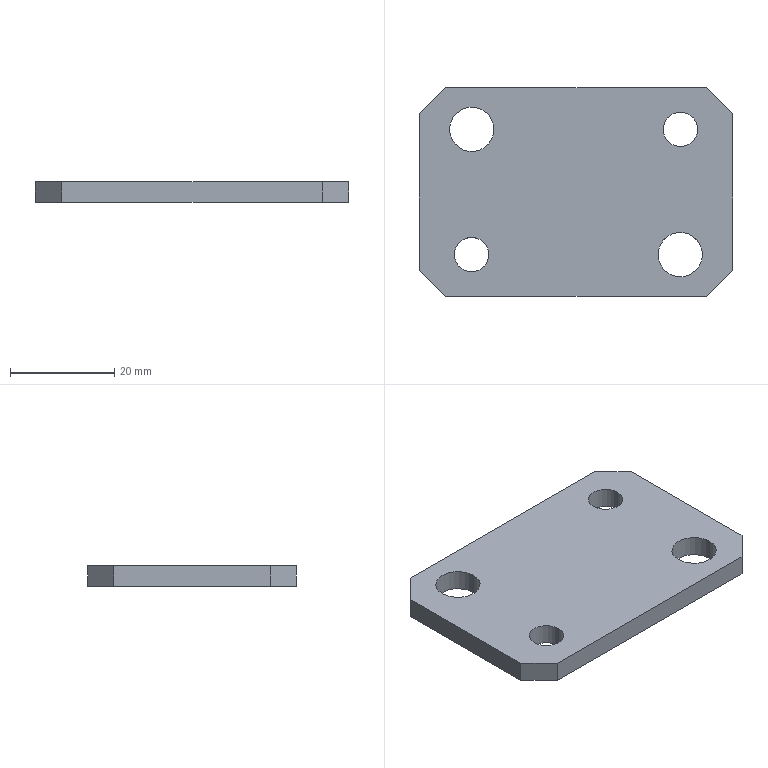Part | SolidWorks | features Chamfer 1, Extrusion 1 | 1 solid | 18 faces | box 60 x 40 x 4 mm | volume 8672 mm3 | plane 10 | cylinder 8 | commonest cylinder face diameters 6.6 x4 8.5 x4
STEP:
#1=CARTESIAN_POINT('',(-18.291,-17.534,4.));
#2=VERTEX_POINT('',#1);
#3=CARTESIAN_POINT('',(-11.691,-17.534,4.));
#4=VERTEX_POINT('',#3);
#5=CARTESIAN_POINT('',(-14.991,-17.534,4.));
#6=DIRECTION('',(0.,0.,1.));
#7=DIRECTION('',(1.,0.,0.));
#8=AXIS2_PLACEMENT_3D('',#5,#6,#7);
#9=CIRCLE('',#8,3.3);
#10=EDGE_CURVE('',#2,#4,#9,.T.);
#11=ORIENTED_EDGE('',*,*,#10,.T.);
#12=CARTESIAN_POINT('',(-11.691,-17.534,0.));
#13=VERTEX_POINT('',#12);
#14=CARTESIAN_POINT('',(-11.691,-17.534,4.));
#15=DIRECTION('',(0.,0.,-1.));
#16=VECTOR('',#15,1000.);
#17=LINE('',#14,#16);
#18=EDGE_CURVE('',#4,#13,#17,.T.);
#19=ORIENTED_EDGE('',*,*,#18,.T.);
#20=CARTESIAN_POINT('',(-18.291,-17.534,0.));
#21=VERTEX_POINT('',#20);
#22=CARTESIAN_POINT('',(-14.991,-17.534,0.));
#23=DIRECTION('',(0.,0.,1.));
#24=DIRECTION('',(1.,0.,0.));
#25=AXIS2_PLACEMENT_3D('',#22,#23,#24);
#26=CIRCLE('',#25,3.3);
#27=EDGE_CURVE('',#21,#13,#26,.T.);
#28=ORIENTED_EDGE('',*,*,#27,.F.);
#29=CARTESIAN_POINT('',(-18.291,-17.534,4.));
#30=DIRECTION('',(0.,0.,-1.));
#31=VECTOR('',#30,1000.);
#32=LINE('',#29,#31);
#33=EDGE_CURVE('',#2,#21,#32,.T.);
#34=ORIENTED_EDGE('',*,*,#33,.F.);
#35=EDGE_LOOP('',(#11,#19,#28,#34));
#36=FACE_OUTER_BOUND('',#35,.T.);
#37=CARTESIAN_POINT('',(-14.991,-17.534,4.));
#38=DIRECTION('',(0.,0.,-1.));
#39=DIRECTION('',(-1.,0.,0.));
#40=AXIS2_PLACEMENT_3D('',#37,#38,#39);
#41=CYLINDRICAL_SURFACE('',#40,3.3);
#42=ADVANCED_FACE('',(#36),#41,.F.);
#43=CARTESIAN_POINT('',(21.709,6.466,4.));
#44=VERTEX_POINT('',#43);
#45=CARTESIAN_POINT('',(28.309,6.466,4.));
#46=VERTEX_POINT('',#45);
#47=CARTESIAN_POINT('',(25.009,6.466,4.));
#48=DIRECTION('',(0.,0.,1.));
#49=DIRECTION('',(1.,0.,0.));
#50=AXIS2_PLACEMENT_3D('',#47,#48,#49);
#51=CIRCLE('',#50,3.3);
#52=EDGE_CURVE('',#44,#46,#51,.T.);
#53=ORIENTED_EDGE('',*,*,#52,.T.);
#54=CARTESIAN_POINT('',(28.309,6.466,0.));
#55=VERTEX_POINT('',#54);
#56=CARTESIAN_POINT('',(28.309,6.466,4.));
#57=DIRECTION('',(0.,0.,-1.));
#58=VECTOR('',#57,1000.);
#59=LINE('',#56,#58);
#60=EDGE_CURVE('',#46,#55,#59,.T.);
#61=ORIENTED_EDGE('',*,*,#60,.T.);
#62=CARTESIAN_POINT('',(21.709,6.466,0.));
#63=VERTEX_POINT('',#62);
#64=CARTESIAN_POINT('',(25.009,6.466,0.));
#65=DIRECTION('',(0.,0.,1.));
#66=DIRECTION('',(1.,0.,0.));
#67=AXIS2_PLACEMENT_3D('',#64,#65,#66);
#68=CIRCLE('',#67,3.3);
#69=EDGE_CURVE('',#63,#55,#68,.T.);
#70=ORIENTED_EDGE('',*,*,#69,.F.);
#71=CARTESIAN_POINT('',(21.709,6.466,4.));
#72=DIRECTION('',(0.,0.,-1.));
#73=VECTOR('',#72,1000.);
#74=LINE('',#71,#73);
#75=EDGE_CURVE('',#44,#63,#74,.T.);
#76=ORIENTED_EDGE('',*,*,#75,.F.);
#77=EDGE_LOOP('',(#53,#61,#70,#76));
#78=FACE_OUTER_BOUND('',#77,.T.);
#79=CARTESIAN_POINT('',(25.009,6.466,4.));
#80=DIRECTION('',(0.,0.,-1.));
#81=DIRECTION('',(-1.,0.,0.));
#82=AXIS2_PLACEMENT_3D('',#79,#80,#81);
#83=CYLINDRICAL_SURFACE('',#82,3.3);
#84=ADVANCED_FACE('',(#78),#83,.F.);
#85=CARTESIAN_POINT('',(20.759,-17.534,4.));
#86=VERTEX_POINT('',#85);
#87=CARTESIAN_POINT('',(29.259,-17.534,4.));
#88=VERTEX_POINT('',#87);
#89=CARTESIAN_POINT('',(25.009,-17.534,4.));
#90=DIRECTION('',(0.,0.,1.));
#91=DIRECTION('',(1.,0.,0.));
#92=AXIS2_PLACEMENT_3D('',#89,#90,#91);
#93=CIRCLE('',#92,4.25);
#94=EDGE_CURVE('',#86,#88,#93,.T.);
#95=ORIENTED_EDGE('',*,*,#94,.T.);
#96=CARTESIAN_POINT('',(29.259,-17.534,0.));
#97=VERTEX_POINT('',#96);
#98=CARTESIAN_POINT('',(29.259,-17.534,4.));
#99=DIRECTION('',(0.,0.,-1.));
#100=VECTOR('',#99,1000.);
#101=LINE('',#98,#100);
#102=EDGE_CURVE('',#88,#97,#101,.T.);
#103=ORIENTED_EDGE('',*,*,#102,.T.);
#104=CARTESIAN_POINT('',(20.759,-17.534,0.));
#105=VERTEX_POINT('',#104);
#106=CARTESIAN_POINT('',(25.009,-17.534,0.));
#107=DIRECTION('',(0.,0.,1.));
#108=DIRECTION('',(1.,0.,0.));
#109=AXIS2_PLACEMENT_3D('',#106,#107,#108);
#110=CIRCLE('',#109,4.25);
#111=EDGE_CURVE('',#105,#97,#110,.T.);
#112=ORIENTED_EDGE('',*,*,#111,.F.);
#113=CARTESIAN_POINT('',(20.759,-17.534,4.));
#114=DIRECTION('',(0.,0.,-1.));
#115=VECTOR('',#114,1000.);
#116=LINE('',#113,#115);
#117=EDGE_CURVE('',#86,#105,#116,.T.);
#118=ORIENTED_EDGE('',*,*,#117,.F.);
#119=EDGE_LOOP('',(#95,#103,#112,#118));
#120=FACE_OUTER_BOUND('',#119,.T.);
#121=CARTESIAN_POINT('',(25.009,-17.534,4.));
#122=DIRECTION('',(0.,0.,-1.));
#123=DIRECTION('',(-1.,0.,0.));
#124=AXIS2_PLACEMENT_3D('',#121,#122,#123);
#125=CYLINDRICAL_SURFACE('',#124,4.25);
#126=ADVANCED_FACE('',(#120),#125,.F.);
#127=CARTESIAN_POINT('',(-19.241,6.466,4.));
#128=VERTEX_POINT('',#127);
#129=CARTESIAN_POINT('',(-10.741,6.466,4.));
#130=VERTEX_POINT('',#129);
#131=CARTESIAN_POINT('',(-14.991,6.466,4.));
#132=DIRECTION('',(0.,0.,1.));
#133=DIRECTION('',(1.,0.,0.));
#134=AXIS2_PLACEMENT_3D('',#131,#132,#133);
#135=CIRCLE('',#134,4.25);
#136=EDGE_CURVE('',#128,#130,#135,.T.);
#137=ORIENTED_EDGE('',*,*,#136,.T.);
#138=CARTESIAN_POINT('',(-10.741,6.466,0.));
#139=VERTEX_POINT('',#138);
#140=CARTESIAN_POINT('',(-10.741,6.466,4.));
#141=DIRECTION('',(0.,0.,-1.));
#142=VECTOR('',#141,1000.);
#143=LINE('',#140,#142);
#144=EDGE_CURVE('',#130,#139,#143,.T.);
#145=ORIENTED_EDGE('',*,*,#144,.T.);
#146=CARTESIAN_POINT('',(-19.241,6.466,0.));
#147=VERTEX_POINT('',#146);
#148=CARTESIAN_POINT('',(-14.991,6.466,0.));
#149=DIRECTION('',(0.,0.,1.));
#150=DIRECTION('',(1.,0.,0.));
#151=AXIS2_PLACEMENT_3D('',#148,#149,#150);
#152=CIRCLE('',#151,4.25);
#153=EDGE_CURVE('',#147,#139,#152,.T.);
#154=ORIENTED_EDGE('',*,*,#153,.F.);
#155=CARTESIAN_POINT('',(-19.241,6.466,4.));
#156=DIRECTION('',(0.,0.,-1.));
#157=VECTOR('',#156,1000.);
#158=LINE('',#155,#157);
#159=EDGE_CURVE('',#128,#147,#158,.T.);
#160=ORIENTED_EDGE('',*,*,#159,.F.);
#161=EDGE_LOOP('',(#137,#145,#154,#160));
#162=FACE_OUTER_BOUND('',#161,.T.);
#163=CARTESIAN_POINT('',(-14.991,6.466,4.));
#164=DIRECTION('',(0.,0.,-1.));
#165=DIRECTION('',(-1.,0.,0.));
#166=AXIS2_PLACEMENT_3D('',#163,#164,#165);
#167=CYLINDRICAL_SURFACE('',#166,4.25);
#168=ADVANCED_FACE('',(#162),#167,.F.);
#169=ORIENTED_EDGE('',*,*,#52,.F.);
#170=CARTESIAN_POINT('',(25.009,6.466,4.));
#171=DIRECTION('',(0.,0.,1.));
#172=DIRECTION('',(1.,0.,0.));
#173=AXIS2_PLACEMENT_3D('',#170,#171,#172);
#174=CIRCLE('',#173,3.3);
#175=EDGE_CURVE('',#46,#44,#174,.T.);
#176=ORIENTED_EDGE('',*,*,#175,.F.);
#177=EDGE_LOOP('',(#169,#176));
#178=FACE_BOUND('',#177,.T.);
#179=ORIENTED_EDGE('',*,*,#136,.F.);
#180=CARTESIAN_POINT('',(-14.991,6.466,4.));
#181=DIRECTION('',(0.,0.,1.));
#182=DIRECTION('',(1.,0.,0.));
#183=AXIS2_PLACEMENT_3D('',#180,#181,#182);
#184=CIRCLE('',#183,4.25);
#185=EDGE_CURVE('',#130,#128,#184,.T.);
#186=ORIENTED_EDGE('',*,*,#185,.F.);
#187=EDGE_LOOP('',(#179,#186));
#188=FACE_BOUND('',#187,.T.);
#189=CARTESIAN_POINT('',(35.009,-20.534,4.));
#190=VERTEX_POINT('',#189);
#191=CARTESIAN_POINT('',(35.009,9.466,4.));
#192=VERTEX_POINT('',#191);
#193=CARTESIAN_POINT('',(35.009,14.466,4.));
#194=DIRECTION('',(0.,1.,0.));
#195=VECTOR('',#194,1000.);
#196=LINE('',#193,#195);
#197=EDGE_CURVE('',#190,#192,#196,.T.);
#198=ORIENTED_EDGE('',*,*,#197,.T.);
#199=CARTESIAN_POINT('',(30.009,14.466,4.));
#200=VERTEX_POINT('',#199);
#201=CARTESIAN_POINT('',(22.238,22.238,4.));
#202=DIRECTION('',(-0.7071,0.7071,0.));
#203=VECTOR('',#202,1000.);
#204=LINE('',#201,#203);
#205=EDGE_CURVE('',#192,#200,#204,.T.);
#206=ORIENTED_EDGE('',*,*,#205,.T.);
#207=CARTESIAN_POINT('',(-19.991,14.466,4.));
#208=VERTEX_POINT('',#207);
#209=CARTESIAN_POINT('',(-24.991,14.466,4.));
#210=DIRECTION('',(-1.,0.,0.));
#211=VECTOR('',#210,1000.);
#212=LINE('',#209,#211);
#213=EDGE_CURVE('',#200,#208,#212,.T.);
#214=ORIENTED_EDGE('',*,*,#213,.T.);
#215=CARTESIAN_POINT('',(-24.991,9.466,4.));
#216=VERTEX_POINT('',#215);
#217=CARTESIAN_POINT('',(-17.228,17.228,4.));
#218=DIRECTION('',(-0.7071,-0.7071,0.));
#219=VECTOR('',#218,1000.);
#220=LINE('',#217,#219);
#221=EDGE_CURVE('',#208,#216,#220,.T.);
#222=ORIENTED_EDGE('',*,*,#221,.T.);
#223=CARTESIAN_POINT('',(-24.991,-20.534,4.));
#224=VERTEX_POINT('',#223);
#225=CARTESIAN_POINT('',(-24.991,14.466,4.));
#226=DIRECTION('',(0.,-1.,0.));
#227=VECTOR('',#226,1000.);
#228=LINE('',#225,#227);
#229=EDGE_CURVE('',#216,#224,#228,.T.);
#230=ORIENTED_EDGE('',*,*,#229,.T.);
#231=CARTESIAN_POINT('',(-19.991,-25.534,4.));
#232=VERTEX_POINT('',#231);
#233=CARTESIAN_POINT('',(-22.762,-22.762,4.));
#234=DIRECTION('',(0.7071,-0.7071,0.));
#235=VECTOR('',#234,1000.);
#236=LINE('',#233,#235);
#237=EDGE_CURVE('',#224,#232,#236,.T.);
#238=ORIENTED_EDGE('',*,*,#237,.T.);
#239=CARTESIAN_POINT('',(30.009,-25.534,4.));
#240=VERTEX_POINT('',#239);
#241=CARTESIAN_POINT('',(-24.991,-25.534,4.));
#242=DIRECTION('',(1.,0.,0.));
#243=VECTOR('',#242,1000.);
#244=LINE('',#241,#243);
#245=EDGE_CURVE('',#232,#240,#244,.T.);
#246=ORIENTED_EDGE('',*,*,#245,.T.);
#247=CARTESIAN_POINT('',(27.772,-27.772,4.));
#248=DIRECTION('',(0.7071,0.7071,0.));
#249=VECTOR('',#248,1000.);
#250=LINE('',#247,#249);
#251=EDGE_CURVE('',#240,#190,#250,.T.);
#252=ORIENTED_EDGE('',*,*,#251,.T.);
#253=EDGE_LOOP('',(#198,#206,#214,#222,#230,#238,#246,#252));
#254=FACE_OUTER_BOUND('',#253,.T.);
#255=ORIENTED_EDGE('',*,*,#94,.F.);
#256=CARTESIAN_POINT('',(25.009,-17.534,4.));
#257=DIRECTION('',(0.,0.,1.));
#258=DIRECTION('',(1.,0.,0.));
#259=AXIS2_PLACEMENT_3D('',#256,#257,#258);
#260=CIRCLE('',#259,4.25);
#261=EDGE_CURVE('',#88,#86,#260,.T.);
#262=ORIENTED_EDGE('',*,*,#261,.F.);
#263=EDGE_LOOP('',(#255,#262));
#264=FACE_BOUND('',#263,.T.);
#265=ORIENTED_EDGE('',*,*,#10,.F.);
#266=CARTESIAN_POINT('',(-14.991,-17.534,4.));
#267=DIRECTION('',(0.,0.,1.));
#268=DIRECTION('',(1.,0.,0.));
#269=AXIS2_PLACEMENT_3D('',#266,#267,#268);
#270=CIRCLE('',#269,3.3);
#271=EDGE_CURVE('',#4,#2,#270,.T.);
#272=ORIENTED_EDGE('',*,*,#271,.F.);
#273=EDGE_LOOP('',(#265,#272));
#274=FACE_BOUND('',#273,.T.);
#275=CARTESIAN_POINT('',(0.,0.,4.));
#276=DIRECTION('',(0.,0.,1.));
#277=DIRECTION('',(1.,0.,0.));
#278=AXIS2_PLACEMENT_3D('',#275,#276,#277);
#279=PLANE('',#278);
#280=ADVANCED_FACE('',(#178,#188,#254,#264,#274),#279,.T.);
#281=CARTESIAN_POINT('',(30.009,14.466,0.));
#282=VERTEX_POINT('',#281);
#283=CARTESIAN_POINT('',(-19.991,14.466,0.));
#284=VERTEX_POINT('',#283);
#285=CARTESIAN_POINT('',(-24.991,14.466,0.));
#286=DIRECTION('',(-1.,0.,0.));
#287=VECTOR('',#286,1000.);
#288=LINE('',#285,#287);
#289=EDGE_CURVE('',#282,#284,#288,.T.);
#290=ORIENTED_EDGE('',*,*,#289,.F.);
#291=CARTESIAN_POINT('',(35.009,9.466,0.));
#292=VERTEX_POINT('',#291);
#293=CARTESIAN_POINT('',(30.009,14.466,0.));
#294=DIRECTION('',(0.7071,-0.7071,0.));
#295=VECTOR('',#294,1000.);
#296=LINE('',#293,#295);
#297=EDGE_CURVE('',#282,#292,#296,.T.);
#298=ORIENTED_EDGE('',*,*,#297,.T.);
#299=CARTESIAN_POINT('',(35.009,-20.534,0.));
#300=VERTEX_POINT('',#299);
#301=CARTESIAN_POINT('',(35.009,14.466,0.));
#302=DIRECTION('',(0.,1.,0.));
#303=VECTOR('',#302,1000.);
#304=LINE('',#301,#303);
#305=EDGE_CURVE('',#300,#292,#304,.T.);
#306=ORIENTED_EDGE('',*,*,#305,.F.);
#307=CARTESIAN_POINT('',(30.009,-25.534,0.));
#308=VERTEX_POINT('',#307);
#309=CARTESIAN_POINT('',(35.009,-20.534,0.));
#310=DIRECTION('',(-0.7071,-0.7071,0.));
#311=VECTOR('',#310,1000.);
#312=LINE('',#309,#311);
#313=EDGE_CURVE('',#300,#308,#312,.T.);
#314=ORIENTED_EDGE('',*,*,#313,.T.);
#315=CARTESIAN_POINT('',(-19.991,-25.534,0.));
#316=VERTEX_POINT('',#315);
#317=CARTESIAN_POINT('',(-24.991,-25.534,0.));
#318=DIRECTION('',(1.,0.,0.));
#319=VECTOR('',#318,1000.);
#320=LINE('',#317,#319);
#321=EDGE_CURVE('',#316,#308,#320,.T.);
#322=ORIENTED_EDGE('',*,*,#321,.F.);
#323=CARTESIAN_POINT('',(-24.991,-20.534,0.));
#324=VERTEX_POINT('',#323);
#325=CARTESIAN_POINT('',(-19.991,-25.534,0.));
#326=DIRECTION('',(-0.7071,0.7071,0.));
#327=VECTOR('',#326,1000.);
#328=LINE('',#325,#327);
#329=EDGE_CURVE('',#316,#324,#328,.T.);
#330=ORIENTED_EDGE('',*,*,#329,.T.);
#331=CARTESIAN_POINT('',(-24.991,9.466,0.));
#332=VERTEX_POINT('',#331);
#333=CARTESIAN_POINT('',(-24.991,14.466,0.));
#334=DIRECTION('',(0.,-1.,0.));
#335=VECTOR('',#334,1000.);
#336=LINE('',#333,#335);
#337=EDGE_CURVE('',#332,#324,#336,.T.);
#338=ORIENTED_EDGE('',*,*,#337,.F.);
#339=CARTESIAN_POINT('',(-24.991,9.466,0.));
#340=DIRECTION('',(0.7071,0.7071,0.));
#341=VECTOR('',#340,1000.);
#342=LINE('',#339,#341);
#343=EDGE_CURVE('',#332,#284,#342,.T.);
#344=ORIENTED_EDGE('',*,*,#343,.T.);
#345=EDGE_LOOP('',(#290,#298,#306,#314,#322,#330,#338,#344));
#346=FACE_OUTER_BOUND('',#345,.T.);
#347=ORIENTED_EDGE('',*,*,#153,.T.);
#348=CARTESIAN_POINT('',(-14.991,6.466,0.));
#349=DIRECTION('',(0.,0.,1.));
#350=DIRECTION('',(1.,0.,0.));
#351=AXIS2_PLACEMENT_3D('',#348,#349,#350);
#352=CIRCLE('',#351,4.25);
#353=EDGE_CURVE('',#139,#147,#352,.T.);
#354=ORIENTED_EDGE('',*,*,#353,.T.);
#355=EDGE_LOOP('',(#347,#354));
#356=FACE_BOUND('',#355,.T.);
#357=ORIENTED_EDGE('',*,*,#111,.T.);
#358=CARTESIAN_POINT('',(25.009,-17.534,0.));
#359=DIRECTION('',(0.,0.,1.));
#360=DIRECTION('',(1.,0.,0.));
#361=AXIS2_PLACEMENT_3D('',#358,#359,#360);
#362=CIRCLE('',#361,4.25);
#363=EDGE_CURVE('',#97,#105,#362,.T.);
#364=ORIENTED_EDGE('',*,*,#363,.T.);
#365=EDGE_LOOP('',(#357,#364));
#366=FACE_BOUND('',#365,.T.);
#367=ORIENTED_EDGE('',*,*,#69,.T.);
#368=CARTESIAN_POINT('',(25.009,6.466,0.));
#369=DIRECTION('',(0.,0.,1.));
#370=DIRECTION('',(1.,0.,0.));
#371=AXIS2_PLACEMENT_3D('',#368,#369,#370);
#372=CIRCLE('',#371,3.3);
#373=EDGE_CURVE('',#55,#63,#372,.T.);
#374=ORIENTED_EDGE('',*,*,#373,.T.);
#375=EDGE_LOOP('',(#367,#374));
#376=FACE_BOUND('',#375,.T.);
#377=ORIENTED_EDGE('',*,*,#27,.T.);
#378=CARTESIAN_POINT('',(-14.991,-17.534,0.));
#379=DIRECTION('',(0.,0.,1.));
#380=DIRECTION('',(1.,0.,0.));
#381=AXIS2_PLACEMENT_3D('',#378,#379,#380);
#382=CIRCLE('',#381,3.3);
#383=EDGE_CURVE('',#13,#21,#382,.T.);
#384=ORIENTED_EDGE('',*,*,#383,.T.);
#385=EDGE_LOOP('',(#377,#384));
#386=FACE_BOUND('',#385,.T.);
#387=CARTESIAN_POINT('',(0.,0.,0.));
#388=DIRECTION('',(0.,0.,1.));
#389=DIRECTION('',(1.,0.,0.));
#390=AXIS2_PLACEMENT_3D('',#387,#388,#389);
#391=PLANE('',#390);
#392=ADVANCED_FACE('',(#346,#356,#366,#376,#386),#391,.F.);
#393=ORIENTED_EDGE('',*,*,#337,.T.);
#394=CARTESIAN_POINT('',(-24.991,-20.534,4.));
#395=DIRECTION('',(0.,0.,1.));
#396=VECTOR('',#395,1000.);
#397=LINE('',#394,#396);
#398=EDGE_CURVE('',#324,#224,#397,.T.);
#399=ORIENTED_EDGE('',*,*,#398,.T.);
#400=ORIENTED_EDGE('',*,*,#229,.F.);
#401=CARTESIAN_POINT('',(-24.991,9.466,4.));
#402=DIRECTION('',(0.,0.,-1.));
#403=VECTOR('',#402,1000.);
#404=LINE('',#401,#403);
#405=EDGE_CURVE('',#216,#332,#404,.T.);
#406=ORIENTED_EDGE('',*,*,#405,.T.);
#407=EDGE_LOOP('',(#393,#399,#400,#406));
#408=FACE_OUTER_BOUND('',#407,.T.);
#409=CARTESIAN_POINT('',(-24.991,14.466,4.));
#410=DIRECTION('',(1.,0.,0.));
#411=DIRECTION('',(0.,1.,0.));
#412=AXIS2_PLACEMENT_3D('',#409,#410,#411);
#413=PLANE('',#412);
#414=ADVANCED_FACE('',(#408),#413,.F.);
#415=ORIENTED_EDGE('',*,*,#321,.T.);
#416=CARTESIAN_POINT('',(30.009,-25.534,4.));
#417=DIRECTION('',(0.,0.,1.));
#418=VECTOR('',#417,1000.);
#419=LINE('',#416,#418);
#420=EDGE_CURVE('',#308,#240,#419,.T.);
#421=ORIENTED_EDGE('',*,*,#420,.T.);
#422=ORIENTED_EDGE('',*,*,#245,.F.);
#423=CARTESIAN_POINT('',(-19.991,-25.534,4.));
#424=DIRECTION('',(0.,0.,-1.));
#425=VECTOR('',#424,1000.);
#426=LINE('',#423,#425);
#427=EDGE_CURVE('',#232,#316,#426,.T.);
#428=ORIENTED_EDGE('',*,*,#427,.T.);
#429=EDGE_LOOP('',(#415,#421,#422,#428));
#430=FACE_OUTER_BOUND('',#429,.T.);
#431=CARTESIAN_POINT('',(-24.991,-25.534,4.));
#432=DIRECTION('',(0.,1.,0.));
#433=DIRECTION('',(0.,0.,1.));
#434=AXIS2_PLACEMENT_3D('',#431,#432,#433);
#435=PLANE('',#434);
#436=ADVANCED_FACE('',(#430),#435,.F.);
#437=ORIENTED_EDGE('',*,*,#305,.T.);
#438=CARTESIAN_POINT('',(35.009,9.466,4.));
#439=DIRECTION('',(0.,0.,1.));
#440=VECTOR('',#439,1000.);
#441=LINE('',#438,#440);
#442=EDGE_CURVE('',#292,#192,#441,.T.);
#443=ORIENTED_EDGE('',*,*,#442,.T.);
#444=ORIENTED_EDGE('',*,*,#197,.F.);
#445=CARTESIAN_POINT('',(35.009,-20.534,4.));
#446=DIRECTION('',(0.,0.,-1.));
#447=VECTOR('',#446,1000.);
#448=LINE('',#445,#447);
#449=EDGE_CURVE('',#190,#300,#448,.T.);
#450=ORIENTED_EDGE('',*,*,#449,.T.);
#451=EDGE_LOOP('',(#437,#443,#444,#450));
#452=FACE_OUTER_BOUND('',#451,.T.);
#453=CARTESIAN_POINT('',(35.009,14.466,4.));
#454=DIRECTION('',(-1.,0.,0.));
#455=DIRECTION('',(0.,0.,1.));
#456=AXIS2_PLACEMENT_3D('',#453,#454,#455);
#457=PLANE('',#456);
#458=ADVANCED_FACE('',(#452),#457,.F.);
#459=ORIENTED_EDGE('',*,*,#213,.F.);
#460=CARTESIAN_POINT('',(30.009,14.466,4.));
#461=DIRECTION('',(0.,0.,-1.));
#462=VECTOR('',#461,1000.);
#463=LINE('',#460,#462);
#464=EDGE_CURVE('',#200,#282,#463,.T.);
#465=ORIENTED_EDGE('',*,*,#464,.T.);
#466=ORIENTED_EDGE('',*,*,#289,.T.);
#467=CARTESIAN_POINT('',(-19.991,14.466,4.));
#468=DIRECTION('',(0.,0.,1.));
#469=VECTOR('',#468,1000.);
#470=LINE('',#467,#469);
#471=EDGE_CURVE('',#284,#208,#470,.T.);
#472=ORIENTED_EDGE('',*,*,#471,.T.);
#473=EDGE_LOOP('',(#459,#465,#466,#472));
#474=FACE_OUTER_BOUND('',#473,.T.);
#475=CARTESIAN_POINT('',(-24.991,14.466,4.));
#476=DIRECTION('',(0.,-1.,0.));
#477=DIRECTION('',(0.,0.,-1.));
#478=AXIS2_PLACEMENT_3D('',#475,#476,#477);
#479=PLANE('',#478);
#480=ADVANCED_FACE('',(#474),#479,.F.);
#481=ORIENTED_EDGE('',*,*,#144,.F.);
#482=ORIENTED_EDGE('',*,*,#185,.T.);
#483=ORIENTED_EDGE('',*,*,#159,.T.);
#484=ORIENTED_EDGE('',*,*,#353,.F.);
#485=EDGE_LOOP('',(#481,#482,#483,#484));
#486=FACE_OUTER_BOUND('',#485,.T.);
#487=CARTESIAN_POINT('',(-14.991,6.466,4.));
#488=DIRECTION('',(0.,0.,-1.));
#489=DIRECTION('',(-1.,0.,0.));
#490=AXIS2_PLACEMENT_3D('',#487,#488,#489);
#491=CYLINDRICAL_SURFACE('',#490,4.25);
#492=ADVANCED_FACE('',(#486),#491,.F.);
#493=ORIENTED_EDGE('',*,*,#102,.F.);
#494=ORIENTED_EDGE('',*,*,#261,.T.);
#495=ORIENTED_EDGE('',*,*,#117,.T.);
#496=ORIENTED_EDGE('',*,*,#363,.F.);
#497=EDGE_LOOP('',(#493,#494,#495,#496));
#498=FACE_OUTER_BOUND('',#497,.T.);
#499=CARTESIAN_POINT('',(25.009,-17.534,4.));
#500=DIRECTION('',(0.,0.,-1.));
#501=DIRECTION('',(-1.,0.,0.));
#502=AXIS2_PLACEMENT_3D('',#499,#500,#501);
#503=CYLINDRICAL_SURFACE('',#502,4.25);
#504=ADVANCED_FACE('',(#498),#503,.F.);
#505=ORIENTED_EDGE('',*,*,#60,.F.);
#506=ORIENTED_EDGE('',*,*,#175,.T.);
#507=ORIENTED_EDGE('',*,*,#75,.T.);
#508=ORIENTED_EDGE('',*,*,#373,.F.);
#509=EDGE_LOOP('',(#505,#506,#507,#508));
#510=FACE_OUTER_BOUND('',#509,.T.);
#511=CARTESIAN_POINT('',(25.009,6.466,4.));
#512=DIRECTION('',(0.,0.,-1.));
#513=DIRECTION('',(-1.,0.,0.));
#514=AXIS2_PLACEMENT_3D('',#511,#512,#513);
#515=CYLINDRICAL_SURFACE('',#514,3.3);
#516=ADVANCED_FACE('',(#510),#515,.F.);
#517=ORIENTED_EDGE('',*,*,#18,.F.);
#518=ORIENTED_EDGE('',*,*,#271,.T.);
#519=ORIENTED_EDGE('',*,*,#33,.T.);
#520=ORIENTED_EDGE('',*,*,#383,.F.);
#521=EDGE_LOOP('',(#517,#518,#519,#520));
#522=FACE_OUTER_BOUND('',#521,.T.);
#523=CARTESIAN_POINT('',(-14.991,-17.534,4.));
#524=DIRECTION('',(0.,0.,-1.));
#525=DIRECTION('',(-1.,0.,0.));
#526=AXIS2_PLACEMENT_3D('',#523,#524,#525);
#527=CYLINDRICAL_SURFACE('',#526,3.3);
#528=ADVANCED_FACE('',(#522),#527,.F.);
#529=ORIENTED_EDGE('',*,*,#205,.F.);
#530=ORIENTED_EDGE('',*,*,#442,.F.);
#531=ORIENTED_EDGE('',*,*,#297,.F.);
#532=ORIENTED_EDGE('',*,*,#464,.F.);
#533=EDGE_LOOP('',(#529,#530,#531,#532));
#534=FACE_OUTER_BOUND('',#533,.T.);
#535=CARTESIAN_POINT('',(30.009,14.466,4.));
#536=DIRECTION('',(-0.7071,-0.7071,0.));
#537=DIRECTION('',(0.,0.,-1.));
#538=AXIS2_PLACEMENT_3D('',#535,#536,#537);
#539=PLANE('',#538);
#540=ADVANCED_FACE('',(#534),#539,.F.);
#541=ORIENTED_EDGE('',*,*,#251,.F.);
#542=ORIENTED_EDGE('',*,*,#420,.F.);
#543=ORIENTED_EDGE('',*,*,#313,.F.);
#544=ORIENTED_EDGE('',*,*,#449,.F.);
#545=EDGE_LOOP('',(#541,#542,#543,#544));
#546=FACE_OUTER_BOUND('',#545,.T.);
#547=CARTESIAN_POINT('',(35.009,-20.534,4.));
#548=DIRECTION('',(-0.7071,0.7071,0.));
#549=DIRECTION('',(0.,0.,-1.));
#550=AXIS2_PLACEMENT_3D('',#547,#548,#549);
#551=PLANE('',#550);
#552=ADVANCED_FACE('',(#546),#551,.F.);
#553=ORIENTED_EDGE('',*,*,#237,.F.);
#554=ORIENTED_EDGE('',*,*,#398,.F.);
#555=ORIENTED_EDGE('',*,*,#329,.F.);
#556=ORIENTED_EDGE('',*,*,#427,.F.);
#557=EDGE_LOOP('',(#553,#554,#555,#556));
#558=FACE_OUTER_BOUND('',#557,.T.);
#559=CARTESIAN_POINT('',(-19.991,-25.534,4.));
#560=DIRECTION('',(0.7071,0.7071,0.));
#561=DIRECTION('',(0.,0.,-1.));
#562=AXIS2_PLACEMENT_3D('',#559,#560,#561);
#563=PLANE('',#562);
#564=ADVANCED_FACE('',(#558),#563,.F.);
#565=ORIENTED_EDGE('',*,*,#221,.F.);
#566=ORIENTED_EDGE('',*,*,#471,.F.);
#567=ORIENTED_EDGE('',*,*,#343,.F.);
#568=ORIENTED_EDGE('',*,*,#405,.F.);
#569=EDGE_LOOP('',(#565,#566,#567,#568));
#570=FACE_OUTER_BOUND('',#569,.T.);
#571=CARTESIAN_POINT('',(-24.991,9.466,4.));
#572=DIRECTION('',(0.7071,-0.7071,0.));
#573=DIRECTION('',(0.,0.,-1.));
#574=AXIS2_PLACEMENT_3D('',#571,#572,#573);
#575=PLANE('',#574);
#576=ADVANCED_FACE('',(#570),#575,.F.);
#577=CLOSED_SHELL('',(#42,#84,#126,#168,#280,#392,#414,#436,#458,#480,#492,#504,#516,#528,#540,#552,#564,#576));
#578=MANIFOLD_SOLID_BREP('',#577);
#579=CARTESIAN_POINT('',(0.,0.,0.));
#580=DIRECTION('',(0.,0.,1.));
#581=DIRECTION('',(1.,0.,0.));
#582=AXIS2_PLACEMENT_3D('',#579,#580,#581);
#583=(LENGTH_UNIT()NAMED_UNIT(*)SI_UNIT(.MILLI.,.METRE.));
#584=UNCERTAINTY_MEASURE_WITH_UNIT(LENGTH_MEASURE(0.00001),#583,'','');
#585=(NAMED_UNIT(*)PLANE_ANGLE_UNIT()SI_UNIT($,.RADIAN.));
#586=(NAMED_UNIT(*)SI_UNIT($,.STERADIAN.)SOLID_ANGLE_UNIT());
#587=(GEOMETRIC_REPRESENTATION_CONTEXT(3)GLOBAL_UNCERTAINTY_ASSIGNED_CONTEXT((#584))GLOBAL_UNIT_ASSIGNED_CONTEXT((#583,#585,#586))REPRESENTATION_CONTEXT('',''));
#588=ADVANCED_BREP_SHAPE_REPRESENTATION('',(#578,#582),#587);